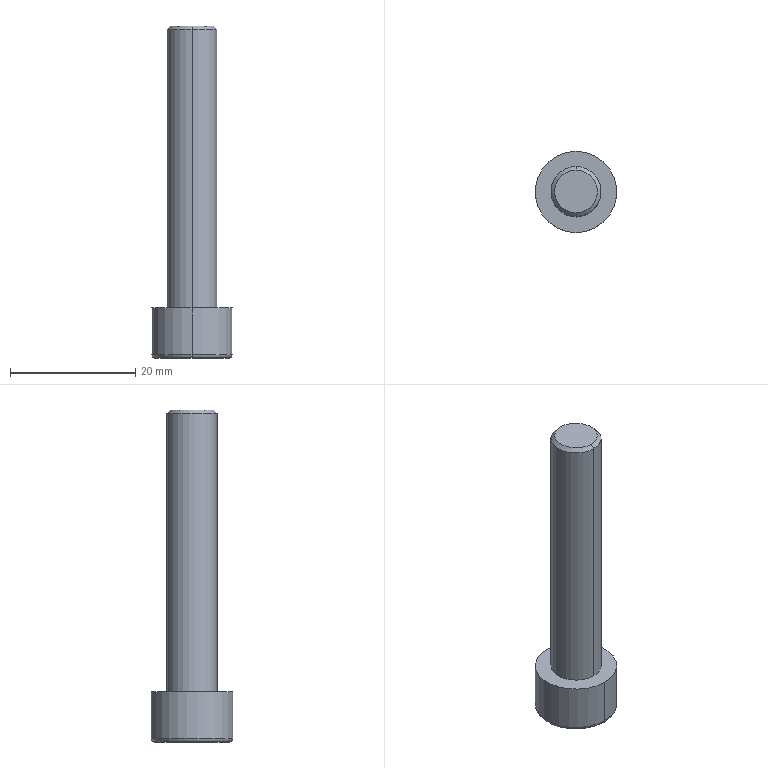Part | Creo | 1 solid | 20 faces | box 13 x 13 x 53 mm | volume 3153 mm3 | plane 10 | torus 4 | cylinder 4 | cone 2 | commonest cylinder face diameters 8 x2 13 x2
STEP:
#1=CARTESIAN_POINT('',(135.,-281.,53.5));
#2=VERTEX_POINT('',#1);
#3=CARTESIAN_POINT('',(135.,-269.,53.5));
#4=VERTEX_POINT('',#3);
#5=CARTESIAN_POINT('',(135.,-275.,53.5));
#6=DIRECTION('',(0.,0.,-1.));
#7=DIRECTION('',(0.,-1.,0.));
#8=AXIS2_PLACEMENT_3D('',#5,#6,#7);
#9=CIRCLE('',#8,6.);
#10=EDGE_CURVE('',#2,#4,#9,.T.);
#11=ORIENTED_EDGE('',*,*,#10,.F.);
#12=CARTESIAN_POINT('',(135.,-275.,53.5));
#13=DIRECTION('',(0.,0.,-1.));
#14=DIRECTION('',(0.,1.,0.));
#15=AXIS2_PLACEMENT_3D('',#12,#13,#14);
#16=CIRCLE('',#15,6.);
#17=EDGE_CURVE('',#4,#2,#16,.T.);
#18=ORIENTED_EDGE('',*,*,#17,.F.);
#19=EDGE_LOOP('',(#11,#18));
#20=FACE_OUTER_BOUND('',#19,.F.);
#21=CARTESIAN_POINT('',(132.,-276.732,53.5));
#22=VERTEX_POINT('',#21);
#23=CARTESIAN_POINT('',(132.,-273.268,53.5));
#24=VERTEX_POINT('',#23);
#25=CARTESIAN_POINT('',(132.,-276.732,53.5));
#26=DIRECTION('',(0.,1.,0.));
#27=VECTOR('',#26,3.464);
#28=LINE('',#25,#27);
#29=EDGE_CURVE('',#22,#24,#28,.T.);
#30=ORIENTED_EDGE('',*,*,#29,.T.);
#31=CARTESIAN_POINT('',(135.,-271.536,53.5));
#32=VERTEX_POINT('',#31);
#33=CARTESIAN_POINT('',(135.,-271.536,53.5));
#34=DIRECTION('',(-0.866,-0.5,0.));
#35=VECTOR('',#34,3.464);
#36=LINE('',#33,#35);
#37=EDGE_CURVE('',#32,#24,#36,.T.);
#38=ORIENTED_EDGE('',*,*,#37,.F.);
#39=CARTESIAN_POINT('',(138.,-273.268,53.5));
#40=VERTEX_POINT('',#39);
#41=CARTESIAN_POINT('',(138.,-273.268,53.5));
#42=DIRECTION('',(-0.866,0.5,0.));
#43=VECTOR('',#42,3.464);
#44=LINE('',#41,#43);
#45=EDGE_CURVE('',#40,#32,#44,.T.);
#46=ORIENTED_EDGE('',*,*,#45,.F.);
#47=CARTESIAN_POINT('',(138.,-276.732,53.5));
#48=VERTEX_POINT('',#47);
#49=CARTESIAN_POINT('',(138.,-273.268,53.5));
#50=DIRECTION('',(0.,-1.,0.));
#51=VECTOR('',#50,3.464);
#52=LINE('',#49,#51);
#53=EDGE_CURVE('',#40,#48,#52,.T.);
#54=ORIENTED_EDGE('',*,*,#53,.T.);
#55=CARTESIAN_POINT('',(135.,-278.464,53.5));
#56=VERTEX_POINT('',#55);
#57=CARTESIAN_POINT('',(135.,-278.464,53.5));
#58=DIRECTION('',(0.866,0.5,0.));
#59=VECTOR('',#58,3.464);
#60=LINE('',#57,#59);
#61=EDGE_CURVE('',#56,#48,#60,.T.);
#62=ORIENTED_EDGE('',*,*,#61,.F.);
#63=CARTESIAN_POINT('',(132.,-276.732,53.5));
#64=DIRECTION('',(0.866,-0.5,0.));
#65=VECTOR('',#64,3.464);
#66=LINE('',#63,#65);
#67=EDGE_CURVE('',#22,#56,#66,.T.);
#68=ORIENTED_EDGE('',*,*,#67,.F.);
#69=EDGE_LOOP('',(#30,#38,#46,#54,#62,#68));
#70=FACE_BOUND('',#69,.F.);
#71=CARTESIAN_POINT('',(135.,-275.,53.5));
#72=DIRECTION('',(0.,0.,-1.));
#73=DIRECTION('',(0.,-1.,0.));
#74=AXIS2_PLACEMENT_3D('',#71,#72,#73);
#75=PLANE('',#74);
#76=ADVANCED_FACE('',(#20,#70),#75,.T.);
#77=ORIENTED_EDGE('',*,*,#10,.T.);
#78=CARTESIAN_POINT('',(135.,-268.646,53.646));
#79=VERTEX_POINT('',#78);
#80=CARTESIAN_POINT('',(135.,-269.,54.));
#81=DIRECTION('',(-1.,0.,0.));
#82=DIRECTION('',(0.,0.7071,-0.7071));
#83=AXIS2_PLACEMENT_3D('',#80,#81,#82);
#84=CIRCLE('',#83,0.5);
#85=EDGE_CURVE('',#79,#4,#84,.T.);
#86=ORIENTED_EDGE('',*,*,#85,.F.);
#87=CARTESIAN_POINT('',(135.,-281.354,53.646));
#88=VERTEX_POINT('',#87);
#89=CARTESIAN_POINT('',(135.,-275.,53.646));
#90=DIRECTION('',(0.,0.,-1.));
#91=DIRECTION('',(0.,-1.,0.));
#92=AXIS2_PLACEMENT_3D('',#89,#90,#91);
#93=CIRCLE('',#92,6.354);
#94=EDGE_CURVE('',#88,#79,#93,.T.);
#95=ORIENTED_EDGE('',*,*,#94,.F.);
#96=CARTESIAN_POINT('',(135.,-281.,54.));
#97=DIRECTION('',(1.,0.,0.));
#98=DIRECTION('',(0.,-0.7071,-0.7071));
#99=AXIS2_PLACEMENT_3D('',#96,#97,#98);
#100=CIRCLE('',#99,0.5);
#101=EDGE_CURVE('',#88,#2,#100,.T.);
#102=ORIENTED_EDGE('',*,*,#101,.T.);
#103=EDGE_LOOP('',(#77,#86,#95,#102));
#104=FACE_OUTER_BOUND('',#103,.F.);
#105=CARTESIAN_POINT('',(135.,-275.,54.));
#106=DIRECTION('',(0.,0.,-1.));
#107=DIRECTION('',(0.,-1.,0.));
#108=AXIS2_PLACEMENT_3D('',#105,#106,#107);
#109=TOROIDAL_SURFACE('',#108,6.,0.5);
#110=ADVANCED_FACE('',(#104),#109,.T.);
#111=ORIENTED_EDGE('',*,*,#17,.T.);
#112=ORIENTED_EDGE('',*,*,#101,.F.);
#113=CARTESIAN_POINT('',(135.,-275.,53.646));
#114=DIRECTION('',(0.,0.,-1.));
#115=DIRECTION('',(0.,1.,0.));
#116=AXIS2_PLACEMENT_3D('',#113,#114,#115);
#117=CIRCLE('',#116,6.354);
#118=EDGE_CURVE('',#79,#88,#117,.T.);
#119=ORIENTED_EDGE('',*,*,#118,.F.);
#120=ORIENTED_EDGE('',*,*,#85,.T.);
#121=EDGE_LOOP('',(#111,#112,#119,#120));
#122=FACE_OUTER_BOUND('',#121,.F.);
#123=CARTESIAN_POINT('',(135.,-275.,54.));
#124=DIRECTION('',(0.,0.,-1.));
#125=DIRECTION('',(0.,-1.,0.));
#126=AXIS2_PLACEMENT_3D('',#123,#124,#125);
#127=TOROIDAL_SURFACE('',#126,6.,0.5);
#128=ADVANCED_FACE('',(#122),#127,.T.);
#129=CARTESIAN_POINT('',(135.,-268.5,54.));
#130=VERTEX_POINT('',#129);
#131=CARTESIAN_POINT('',(135.,-281.5,54.));
#132=VERTEX_POINT('',#131);
#133=CARTESIAN_POINT('',(135.,-275.,54.));
#134=DIRECTION('',(0.,0.,-1.));
#135=DIRECTION('',(0.,1.,0.));
#136=AXIS2_PLACEMENT_3D('',#133,#134,#135);
#137=CIRCLE('',#136,6.5);
#138=EDGE_CURVE('',#130,#132,#137,.T.);
#139=ORIENTED_EDGE('',*,*,#138,.F.);
#140=CARTESIAN_POINT('',(135.,-269.,54.));
#141=DIRECTION('',(-1.,0.,0.));
#142=DIRECTION('',(0.,1.,0.));
#143=AXIS2_PLACEMENT_3D('',#140,#141,#142);
#144=CIRCLE('',#143,0.5);
#145=EDGE_CURVE('',#130,#79,#144,.T.);
#146=ORIENTED_EDGE('',*,*,#145,.T.);
#147=ORIENTED_EDGE('',*,*,#118,.T.);
#148=CARTESIAN_POINT('',(135.,-281.,54.));
#149=DIRECTION('',(1.,0.,0.));
#150=DIRECTION('',(0.,-1.,0.));
#151=AXIS2_PLACEMENT_3D('',#148,#149,#150);
#152=CIRCLE('',#151,0.5);
#153=EDGE_CURVE('',#132,#88,#152,.T.);
#154=ORIENTED_EDGE('',*,*,#153,.F.);
#155=EDGE_LOOP('',(#139,#146,#147,#154));
#156=FACE_OUTER_BOUND('',#155,.F.);
#157=CARTESIAN_POINT('',(135.,-275.,54.));
#158=DIRECTION('',(0.,0.,-1.));
#159=DIRECTION('',(0.,-1.,0.));
#160=AXIS2_PLACEMENT_3D('',#157,#158,#159);
#161=TOROIDAL_SURFACE('',#160,6.,0.5);
#162=ADVANCED_FACE('',(#156),#161,.T.);
#163=ORIENTED_EDGE('',*,*,#138,.T.);
#164=CARTESIAN_POINT('',(135.,-281.5,61.5));
#165=VERTEX_POINT('',#164);
#166=CARTESIAN_POINT('',(135.,-281.5,61.5));
#167=DIRECTION('',(0.,0.,-1.));
#168=VECTOR('',#167,7.5);
#169=LINE('',#166,#168);
#170=EDGE_CURVE('',#165,#132,#169,.T.);
#171=ORIENTED_EDGE('',*,*,#170,.F.);
#172=CARTESIAN_POINT('',(135.,-268.5,61.5));
#173=VERTEX_POINT('',#172);
#174=CARTESIAN_POINT('',(135.,-275.,61.5));
#175=DIRECTION('',(0.,0.,1.));
#176=DIRECTION('',(0.,-1.,0.));
#177=AXIS2_PLACEMENT_3D('',#174,#175,#176);
#178=CIRCLE('',#177,6.5);
#179=EDGE_CURVE('',#165,#173,#178,.T.);
#180=ORIENTED_EDGE('',*,*,#179,.T.);
#181=CARTESIAN_POINT('',(135.,-268.5,61.5));
#182=DIRECTION('',(0.,0.,-1.));
#183=VECTOR('',#182,7.5);
#184=LINE('',#181,#183);
#185=EDGE_CURVE('',#173,#130,#184,.T.);
#186=ORIENTED_EDGE('',*,*,#185,.T.);
#187=EDGE_LOOP('',(#163,#171,#180,#186));
#188=FACE_OUTER_BOUND('',#187,.F.);
#189=CARTESIAN_POINT('',(135.,-275.,61.5));
#190=DIRECTION('',(0.,0.,-1.));
#191=DIRECTION('',(0.,-1.,0.));
#192=AXIS2_PLACEMENT_3D('',#189,#190,#191);
#193=CYLINDRICAL_SURFACE('',#192,6.5);
#194=ADVANCED_FACE('',(#188),#193,.T.);
#195=CARTESIAN_POINT('',(135.,-275.,54.));
#196=DIRECTION('',(0.,0.,-1.));
#197=DIRECTION('',(0.,-1.,0.));
#198=AXIS2_PLACEMENT_3D('',#195,#196,#197);
#199=CIRCLE('',#198,6.5);
#200=EDGE_CURVE('',#132,#130,#199,.T.);
#201=ORIENTED_EDGE('',*,*,#200,.T.);
#202=ORIENTED_EDGE('',*,*,#185,.F.);
#203=CARTESIAN_POINT('',(135.,-275.,61.5));
#204=DIRECTION('',(0.,0.,1.));
#205=DIRECTION('',(0.,1.,0.));
#206=AXIS2_PLACEMENT_3D('',#203,#204,#205);
#207=CIRCLE('',#206,6.5);
#208=EDGE_CURVE('',#173,#165,#207,.T.);
#209=ORIENTED_EDGE('',*,*,#208,.T.);
#210=ORIENTED_EDGE('',*,*,#170,.T.);
#211=EDGE_LOOP('',(#201,#202,#209,#210));
#212=FACE_OUTER_BOUND('',#211,.F.);
#213=CARTESIAN_POINT('',(135.,-275.,61.5));
#214=DIRECTION('',(0.,0.,-1.));
#215=DIRECTION('',(0.,-1.,0.));
#216=AXIS2_PLACEMENT_3D('',#213,#214,#215);
#217=CYLINDRICAL_SURFACE('',#216,6.5);
#218=ADVANCED_FACE('',(#212),#217,.T.);
#219=ORIENTED_EDGE('',*,*,#200,.F.);
#220=ORIENTED_EDGE('',*,*,#153,.T.);
#221=ORIENTED_EDGE('',*,*,#94,.T.);
#222=ORIENTED_EDGE('',*,*,#145,.F.);
#223=EDGE_LOOP('',(#219,#220,#221,#222));
#224=FACE_OUTER_BOUND('',#223,.F.);
#225=CARTESIAN_POINT('',(135.,-275.,54.));
#226=DIRECTION('',(0.,0.,-1.));
#227=DIRECTION('',(0.,-1.,0.));
#228=AXIS2_PLACEMENT_3D('',#225,#226,#227);
#229=TOROIDAL_SURFACE('',#228,6.,0.5);
#230=ADVANCED_FACE('',(#224),#229,.T.);
#231=ORIENTED_EDGE('',*,*,#179,.F.);
#232=ORIENTED_EDGE('',*,*,#208,.F.);
#233=EDGE_LOOP('',(#231,#232));
#234=FACE_OUTER_BOUND('',#233,.F.);
#235=CARTESIAN_POINT('',(135.,-279.,61.5));
#236=VERTEX_POINT('',#235);
#237=CARTESIAN_POINT('',(135.,-271.,61.5));
#238=VERTEX_POINT('',#237);
#239=CARTESIAN_POINT('',(135.,-275.,61.5));
#240=DIRECTION('',(0.,0.,-1.));
#241=DIRECTION('',(0.,-1.,0.));
#242=AXIS2_PLACEMENT_3D('',#239,#240,#241);
#243=CIRCLE('',#242,4.);
#244=EDGE_CURVE('',#236,#238,#243,.T.);
#245=ORIENTED_EDGE('',*,*,#244,.F.);
#246=CARTESIAN_POINT('',(135.,-275.,61.5));
#247=DIRECTION('',(0.,0.,-1.));
#248=DIRECTION('',(0.,1.,0.));
#249=AXIS2_PLACEMENT_3D('',#246,#247,#248);
#250=CIRCLE('',#249,4.);
#251=EDGE_CURVE('',#238,#236,#250,.T.);
#252=ORIENTED_EDGE('',*,*,#251,.F.);
#253=EDGE_LOOP('',(#245,#252));
#254=FACE_BOUND('',#253,.F.);
#255=CARTESIAN_POINT('',(135.,-275.,61.5));
#256=DIRECTION('',(0.,0.,1.));
#257=DIRECTION('',(0.,1.,0.));
#258=AXIS2_PLACEMENT_3D('',#255,#256,#257);
#259=PLANE('',#258);
#260=ADVANCED_FACE('',(#234,#254),#259,.T.);
#261=CARTESIAN_POINT('',(135.,-271.,105.9));
#262=VERTEX_POINT('',#261);
#263=CARTESIAN_POINT('',(135.,-279.,105.9));
#264=VERTEX_POINT('',#263);
#265=CARTESIAN_POINT('',(135.,-275.,105.9));
#266=DIRECTION('',(0.,0.,1.));
#267=DIRECTION('',(0.,1.,0.));
#268=AXIS2_PLACEMENT_3D('',#265,#266,#267);
#269=CIRCLE('',#268,4.);
#270=EDGE_CURVE('',#262,#264,#269,.T.);
#271=ORIENTED_EDGE('',*,*,#270,.T.);
#272=CARTESIAN_POINT('',(135.,-279.,105.9));
#273=DIRECTION('',(0.,0.,-1.));
#274=VECTOR('',#273,44.4);
#275=LINE('',#272,#274);
#276=EDGE_CURVE('',#264,#236,#275,.T.);
#277=ORIENTED_EDGE('',*,*,#276,.T.);
#278=ORIENTED_EDGE('',*,*,#244,.T.);
#279=CARTESIAN_POINT('',(135.,-271.,105.9));
#280=DIRECTION('',(0.,0.,-1.));
#281=VECTOR('',#280,44.4);
#282=LINE('',#279,#281);
#283=EDGE_CURVE('',#262,#238,#282,.T.);
#284=ORIENTED_EDGE('',*,*,#283,.F.);
#285=EDGE_LOOP('',(#271,#277,#278,#284));
#286=FACE_OUTER_BOUND('',#285,.F.);
#287=CARTESIAN_POINT('',(135.,-275.,106.5));
#288=DIRECTION('',(0.,0.,-1.));
#289=DIRECTION('',(0.,-1.,0.));
#290=AXIS2_PLACEMENT_3D('',#287,#288,#289);
#291=CYLINDRICAL_SURFACE('',#290,4.);
#292=ADVANCED_FACE('',(#286),#291,.T.);
#293=CARTESIAN_POINT('',(135.,-271.6,106.5));
#294=VERTEX_POINT('',#293);
#295=CARTESIAN_POINT('',(135.,-278.4,106.5));
#296=VERTEX_POINT('',#295);
#297=CARTESIAN_POINT('',(135.,-275.,106.5));
#298=DIRECTION('',(0.,0.,1.));
#299=DIRECTION('',(0.,1.,0.));
#300=AXIS2_PLACEMENT_3D('',#297,#298,#299);
#301=CIRCLE('',#300,3.4);
#302=EDGE_CURVE('',#294,#296,#301,.T.);
#303=ORIENTED_EDGE('',*,*,#302,.T.);
#304=CARTESIAN_POINT('',(135.,-278.4,106.5));
#305=DIRECTION('',(0.,-0.7071,-0.7071));
#306=VECTOR('',#305,0.8485);
#307=LINE('',#304,#306);
#308=EDGE_CURVE('',#296,#264,#307,.T.);
#309=ORIENTED_EDGE('',*,*,#308,.T.);
#310=ORIENTED_EDGE('',*,*,#270,.F.);
#311=CARTESIAN_POINT('',(135.,-271.6,106.5));
#312=DIRECTION('',(0.,0.7071,-0.7071));
#313=VECTOR('',#312,0.8485);
#314=LINE('',#311,#313);
#315=EDGE_CURVE('',#294,#262,#314,.T.);
#316=ORIENTED_EDGE('',*,*,#315,.F.);
#317=EDGE_LOOP('',(#303,#309,#310,#316));
#318=FACE_OUTER_BOUND('',#317,.F.);
#319=CARTESIAN_POINT('',(135.,-275.,106.2));
#320=DIRECTION('',(0.,0.,-1.));
#321=DIRECTION('',(0.,-1.,0.));
#322=AXIS2_PLACEMENT_3D('',#319,#320,#321);
#323=CONICAL_SURFACE('',#322,3.7,45.);
#324=ADVANCED_FACE('',(#318),#323,.T.);
#325=CARTESIAN_POINT('',(135.,-275.,106.5));
#326=DIRECTION('',(0.,0.,1.));
#327=DIRECTION('',(0.,-1.,0.));
#328=AXIS2_PLACEMENT_3D('',#325,#326,#327);
#329=CIRCLE('',#328,3.4);
#330=EDGE_CURVE('',#296,#294,#329,.T.);
#331=ORIENTED_EDGE('',*,*,#330,.F.);
#332=ORIENTED_EDGE('',*,*,#302,.F.);
#333=EDGE_LOOP('',(#331,#332));
#334=FACE_OUTER_BOUND('',#333,.F.);
#335=CARTESIAN_POINT('',(135.,-275.,106.5));
#336=DIRECTION('',(0.,0.,-1.));
#337=DIRECTION('',(0.,-1.,0.));
#338=AXIS2_PLACEMENT_3D('',#335,#336,#337);
#339=PLANE('',#338);
#340=ADVANCED_FACE('',(#334),#339,.F.);
#341=ORIENTED_EDGE('',*,*,#330,.T.);
#342=ORIENTED_EDGE('',*,*,#315,.T.);
#343=CARTESIAN_POINT('',(135.,-275.,105.9));
#344=DIRECTION('',(0.,0.,1.));
#345=DIRECTION('',(0.,-1.,0.));
#346=AXIS2_PLACEMENT_3D('',#343,#344,#345);
#347=CIRCLE('',#346,4.);
#348=EDGE_CURVE('',#264,#262,#347,.T.);
#349=ORIENTED_EDGE('',*,*,#348,.F.);
#350=ORIENTED_EDGE('',*,*,#308,.F.);
#351=EDGE_LOOP('',(#341,#342,#349,#350));
#352=FACE_OUTER_BOUND('',#351,.F.);
#353=CARTESIAN_POINT('',(135.,-275.,106.2));
#354=DIRECTION('',(0.,0.,-1.));
#355=DIRECTION('',(0.,-1.,0.));
#356=AXIS2_PLACEMENT_3D('',#353,#354,#355);
#357=CONICAL_SURFACE('',#356,3.7,45.);
#358=ADVANCED_FACE('',(#352),#357,.T.);
#359=ORIENTED_EDGE('',*,*,#348,.T.);
#360=ORIENTED_EDGE('',*,*,#283,.T.);
#361=ORIENTED_EDGE('',*,*,#251,.T.);
#362=ORIENTED_EDGE('',*,*,#276,.F.);
#363=EDGE_LOOP('',(#359,#360,#361,#362));
#364=FACE_OUTER_BOUND('',#363,.F.);
#365=CARTESIAN_POINT('',(135.,-275.,106.5));
#366=DIRECTION('',(0.,0.,-1.));
#367=DIRECTION('',(0.,-1.,0.));
#368=AXIS2_PLACEMENT_3D('',#365,#366,#367);
#369=CYLINDRICAL_SURFACE('',#368,4.);
#370=ADVANCED_FACE('',(#364),#369,.T.);
#371=ORIENTED_EDGE('',*,*,#29,.F.);
#372=CARTESIAN_POINT('',(132.,-276.732,58.78));
#373=VERTEX_POINT('',#372);
#374=CARTESIAN_POINT('',(132.,-276.732,53.5));
#375=DIRECTION('',(0.,0.,1.));
#376=VECTOR('',#375,5.28);
#377=LINE('',#374,#376);
#378=EDGE_CURVE('',#22,#373,#377,.T.);
#379=ORIENTED_EDGE('',*,*,#378,.T.);
#380=CARTESIAN_POINT('',(132.,-273.268,58.78));
#381=VERTEX_POINT('',#380);
#382=CARTESIAN_POINT('',(132.,-276.732,58.78));
#383=DIRECTION('',(0.,1.,0.));
#384=VECTOR('',#383,3.464);
#385=LINE('',#382,#384);
#386=EDGE_CURVE('',#373,#381,#385,.T.);
#387=ORIENTED_EDGE('',*,*,#386,.T.);
#388=CARTESIAN_POINT('',(132.,-273.268,53.5));
#389=DIRECTION('',(0.,0.,1.));
#390=VECTOR('',#389,5.28);
#391=LINE('',#388,#390);
#392=EDGE_CURVE('',#24,#381,#391,.T.);
#393=ORIENTED_EDGE('',*,*,#392,.F.);
#394=EDGE_LOOP('',(#371,#379,#387,#393));
#395=FACE_OUTER_BOUND('',#394,.F.);
#396=CARTESIAN_POINT('',(132.,-273.268,58.78));
#397=DIRECTION('',(1.,0.,0.));
#398=DIRECTION('',(0.,0.,1.));
#399=AXIS2_PLACEMENT_3D('',#396,#397,#398);
#400=PLANE('',#399);
#401=ADVANCED_FACE('',(#395),#400,.T.);
#402=ORIENTED_EDGE('',*,*,#67,.T.);
#403=CARTESIAN_POINT('',(135.,-278.464,58.78));
#404=VERTEX_POINT('',#403);
#405=CARTESIAN_POINT('',(135.,-278.464,53.5));
#406=DIRECTION('',(0.,0.,1.));
#407=VECTOR('',#406,5.28);
#408=LINE('',#405,#407);
#409=EDGE_CURVE('',#56,#404,#408,.T.);
#410=ORIENTED_EDGE('',*,*,#409,.T.);
#411=CARTESIAN_POINT('',(135.,-278.464,58.78));
#412=DIRECTION('',(-0.866,0.5,0.));
#413=VECTOR('',#412,3.464);
#414=LINE('',#411,#413);
#415=EDGE_CURVE('',#404,#373,#414,.T.);
#416=ORIENTED_EDGE('',*,*,#415,.T.);
#417=ORIENTED_EDGE('',*,*,#378,.F.);
#418=EDGE_LOOP('',(#402,#410,#416,#417));
#419=FACE_OUTER_BOUND('',#418,.F.);
#420=CARTESIAN_POINT('',(132.,-276.732,58.78));
#421=DIRECTION('',(0.5,0.866,0.));
#422=DIRECTION('',(0.866,-0.5,0.));
#423=AXIS2_PLACEMENT_3D('',#420,#421,#422);
#424=PLANE('',#423);
#425=ADVANCED_FACE('',(#419),#424,.T.);
#426=ORIENTED_EDGE('',*,*,#61,.T.);
#427=CARTESIAN_POINT('',(138.,-276.732,58.78));
#428=VERTEX_POINT('',#427);
#429=CARTESIAN_POINT('',(138.,-276.732,53.5));
#430=DIRECTION('',(0.,0.,1.));
#431=VECTOR('',#430,5.28);
#432=LINE('',#429,#431);
#433=EDGE_CURVE('',#48,#428,#432,.T.);
#434=ORIENTED_EDGE('',*,*,#433,.T.);
#435=CARTESIAN_POINT('',(138.,-276.732,58.78));
#436=DIRECTION('',(-0.866,-0.5,0.));
#437=VECTOR('',#436,3.464);
#438=LINE('',#435,#437);
#439=EDGE_CURVE('',#428,#404,#438,.T.);
#440=ORIENTED_EDGE('',*,*,#439,.T.);
#441=ORIENTED_EDGE('',*,*,#409,.F.);
#442=EDGE_LOOP('',(#426,#434,#440,#441));
#443=FACE_OUTER_BOUND('',#442,.F.);
#444=CARTESIAN_POINT('',(135.,-278.464,58.78));
#445=DIRECTION('',(-0.5,0.866,0.));
#446=DIRECTION('',(0.866,0.5,0.));
#447=AXIS2_PLACEMENT_3D('',#444,#445,#446);
#448=PLANE('',#447);
#449=ADVANCED_FACE('',(#443),#448,.T.);
#450=ORIENTED_EDGE('',*,*,#53,.F.);
#451=CARTESIAN_POINT('',(138.,-273.268,58.78));
#452=VERTEX_POINT('',#451);
#453=CARTESIAN_POINT('',(138.,-273.268,53.5));
#454=DIRECTION('',(0.,0.,1.));
#455=VECTOR('',#454,5.28);
#456=LINE('',#453,#455);
#457=EDGE_CURVE('',#40,#452,#456,.T.);
#458=ORIENTED_EDGE('',*,*,#457,.T.);
#459=CARTESIAN_POINT('',(138.,-273.268,58.78));
#460=DIRECTION('',(0.,-1.,0.));
#461=VECTOR('',#460,3.464);
#462=LINE('',#459,#461);
#463=EDGE_CURVE('',#452,#428,#462,.T.);
#464=ORIENTED_EDGE('',*,*,#463,.T.);
#465=ORIENTED_EDGE('',*,*,#433,.F.);
#466=EDGE_LOOP('',(#450,#458,#464,#465));
#467=FACE_OUTER_BOUND('',#466,.F.);
#468=CARTESIAN_POINT('',(138.,-276.732,58.78));
#469=DIRECTION('',(-1.,0.,0.));
#470=DIRECTION('',(0.,0.,-1.));
#471=AXIS2_PLACEMENT_3D('',#468,#469,#470);
#472=PLANE('',#471);
#473=ADVANCED_FACE('',(#467),#472,.T.);
#474=ORIENTED_EDGE('',*,*,#45,.T.);
#475=CARTESIAN_POINT('',(135.,-271.536,58.78));
#476=VERTEX_POINT('',#475);
#477=CARTESIAN_POINT('',(135.,-271.536,53.5));
#478=DIRECTION('',(0.,0.,1.));
#479=VECTOR('',#478,5.28);
#480=LINE('',#477,#479);
#481=EDGE_CURVE('',#32,#476,#480,.T.);
#482=ORIENTED_EDGE('',*,*,#481,.T.);
#483=CARTESIAN_POINT('',(135.,-271.536,58.78));
#484=DIRECTION('',(0.866,-0.5,0.));
#485=VECTOR('',#484,3.464);
#486=LINE('',#483,#485);
#487=EDGE_CURVE('',#476,#452,#486,.T.);
#488=ORIENTED_EDGE('',*,*,#487,.T.);
#489=ORIENTED_EDGE('',*,*,#457,.F.);
#490=EDGE_LOOP('',(#474,#482,#488,#489));
#491=FACE_OUTER_BOUND('',#490,.F.);
#492=CARTESIAN_POINT('',(138.,-273.268,58.78));
#493=DIRECTION('',(-0.5,-0.866,0.));
#494=DIRECTION('',(-0.866,0.5,0.));
#495=AXIS2_PLACEMENT_3D('',#492,#493,#494);
#496=PLANE('',#495);
#497=ADVANCED_FACE('',(#491),#496,.T.);
#498=ORIENTED_EDGE('',*,*,#37,.T.);
#499=ORIENTED_EDGE('',*,*,#392,.T.);
#500=CARTESIAN_POINT('',(132.,-273.268,58.78));
#501=DIRECTION('',(0.866,0.5,0.));
#502=VECTOR('',#501,3.464);
#503=LINE('',#500,#502);
#504=EDGE_CURVE('',#381,#476,#503,.T.);
#505=ORIENTED_EDGE('',*,*,#504,.T.);
#506=ORIENTED_EDGE('',*,*,#481,.F.);
#507=EDGE_LOOP('',(#498,#499,#505,#506));
#508=FACE_OUTER_BOUND('',#507,.F.);
#509=CARTESIAN_POINT('',(135.,-271.536,58.78));
#510=DIRECTION('',(0.5,-0.866,0.));
#511=DIRECTION('',(-0.866,-0.5,0.));
#512=AXIS2_PLACEMENT_3D('',#509,#510,#511);
#513=PLANE('',#512);
#514=ADVANCED_FACE('',(#508),#513,.T.);
#515=ORIENTED_EDGE('',*,*,#415,.F.);
#516=ORIENTED_EDGE('',*,*,#439,.F.);
#517=ORIENTED_EDGE('',*,*,#463,.F.);
#518=ORIENTED_EDGE('',*,*,#487,.F.);
#519=ORIENTED_EDGE('',*,*,#504,.F.);
#520=ORIENTED_EDGE('',*,*,#386,.F.);
#521=EDGE_LOOP('',(#515,#516,#517,#518,#519,#520));
#522=FACE_OUTER_BOUND('',#521,.F.);
#523=CARTESIAN_POINT('',(138.,-280.196,58.78));
#524=DIRECTION('',(0.,0.,1.));
#525=DIRECTION('',(0.,1.,0.));
#526=AXIS2_PLACEMENT_3D('',#523,#524,#525);
#527=PLANE('',#526);
#528=ADVANCED_FACE('',(#522),#527,.F.);
#529=CLOSED_SHELL('',(#76,#110,#128,#162,#194,#218,#230,#260,#292,#324,#340,#358,#370,#401,#425,#449,#473,#497,#514,#528));
#530=MANIFOLD_SOLID_BREP('',#529);
#531=(LENGTH_UNIT()NAMED_UNIT(*)SI_UNIT(.MILLI.,.METRE.));
#532=UNCERTAINTY_MEASURE_WITH_UNIT(LENGTH_MEASURE(0.00561),#531,'','');
#533=(NAMED_UNIT(*)PLANE_ANGLE_UNIT()SI_UNIT($,.RADIAN.));
#534=PLANE_ANGLE_MEASURE_WITH_UNIT(PLANE_ANGLE_MEASURE(0.01745),#533);
#535=(CONVERSION_BASED_UNIT('DEGREE',#534)NAMED_UNIT(*)PLANE_ANGLE_UNIT());
#536=(NAMED_UNIT(*)SI_UNIT($,.STERADIAN.)SOLID_ANGLE_UNIT());
#537=(GEOMETRIC_REPRESENTATION_CONTEXT(3)GLOBAL_UNCERTAINTY_ASSIGNED_CONTEXT((#532))GLOBAL_UNIT_ASSIGNED_CONTEXT((#531,#535,#536))REPRESENTATION_CONTEXT('',''));
#538=ADVANCED_BREP_SHAPE_REPRESENTATION('',(#530),#537);